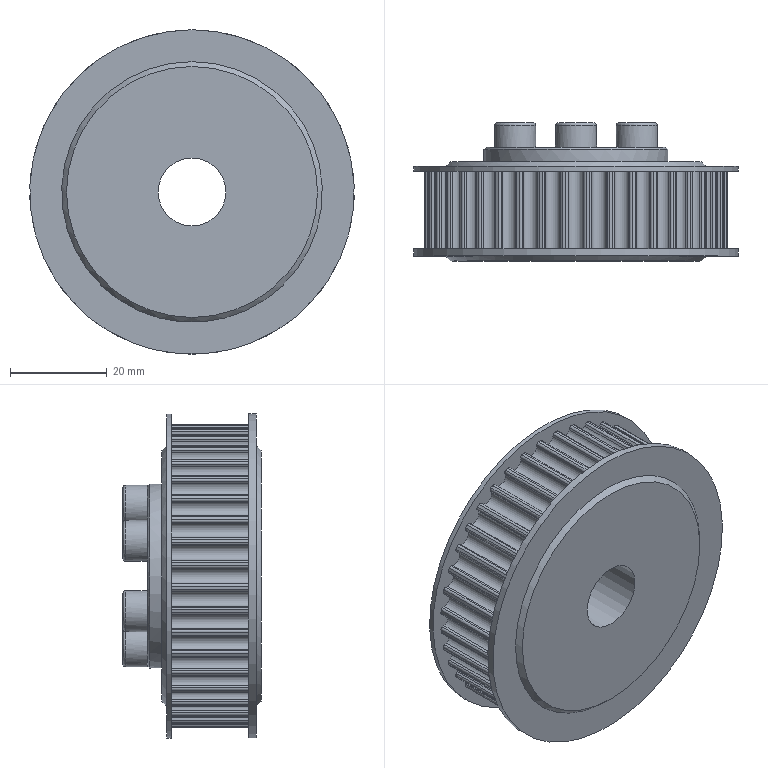Part | STEP file | 冲床-300配套压波_id314_x_t | 1 solid | 338 faces | box 67 x 28.5 x 67 mm | volume 59308 mm3 | cylinder 176 | plane 147 | cone 9 | torus 6 | commonest cylinder face diameters 1 x80 3.12 x40 62.52 x40 4.2 x6 8.5 x6 67 x2